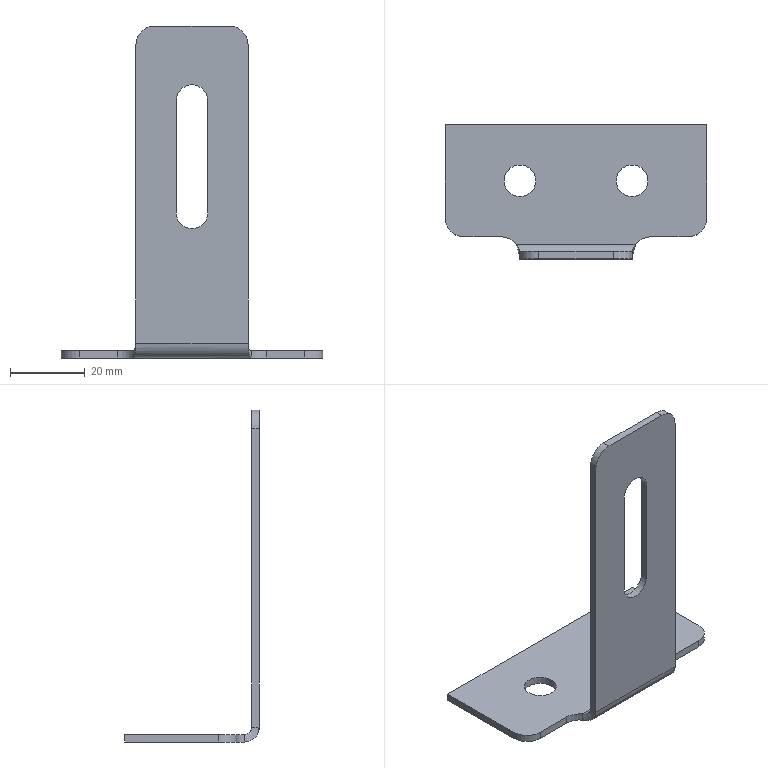Part | STEP file | S1 | 1 solid | 28 faces | box 70 x 36 x 88.858 mm | volume 8824 mm3 | plane 14 | cylinder 12 | spline 2 | commonest cylinder face diameters 10 x6 8.5 x4 4 x1 8 x1